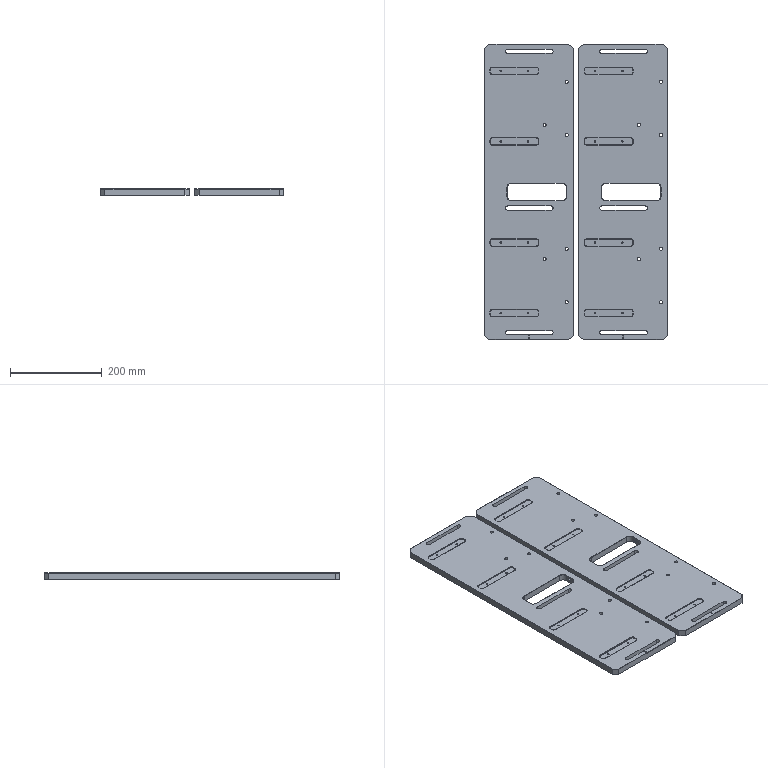NC program | NX | posted by the shop | part box 401 x 645 x 14 mm
Lines 2473 to 4203 of 5636, first 1379 of 1731 lines:
N3 T09 M06
(D10  D=10. R=0. H=09 ce=0.10 di=0.00)
G00 G90 G54 X0.0 Y205.6 M03 S6000
G43 H09 Z34.
M08
Z14.
G01 X312.5 Z13.907 F4000.
G02 X316.106 Y204.106 Z13.906 I0.0 J-5.1
G01 X326.106 Y194.106 Z13.902
G02 X327.6 Y190.5 Z13.901 I-3.606 J-3.606
G01 Y15.5 Z13.849
G02 X326.106 Y11.894 Z13.848 I-5.1 J0.0
G01 X316.106 Y1.894 Z13.844
G02 X312.5 Y.4 Z13.843 I-3.606 J3.606
G01 X-312.5 Z13.657
G02 X-316.106 Y1.894 Z13.656 I0.0 J5.1
G01 X-326.106 Y11.894 Z13.652
G02 X-327.6 Y15.5 Z13.651 I3.606 J3.606
G01 Y190.5 Z13.599
G02 X-327.596 Y190.713 Z13.599 I5.1 J0.0
X-326.106 Y194.106 Z13.598 I5.096 J-.213
G01 X-316.106 Y204.106 Z13.594
G02 X-312.5 Y205.6 Z13.593 I3.606 J-3.606
G01 X312.5 Z13.407
G02 X316.106 Y204.106 Z13.406 I0.0 J-5.1
G01 X326.106 Y194.106 Z13.402
G02 X327.6 Y190.5 Z13.401 I-3.606 J-3.606
G01 Y15.5 Z13.349
G02 X326.106 Y11.894 Z13.348 I-5.1 J0.0
G01 X316.106 Y1.894 Z13.344
G02 X312.5 Y.4 Z13.343 I-3.606 J3.606
G01 X-312.5 Z13.157
G02 X-316.106 Y1.894 Z13.156 I0.0 J5.1
G01 X-326.106 Y11.894 Z13.152
G02 X-327.6 Y15.5 Z13.151 I3.606 J3.606
G01 Y190.5 Z13.099
G02 X-327.596 Y190.713 Z13.099 I5.1 J0.0
X-326.106 Y194.106 Z13.098 I5.096 J-.213
G01 X-316.106 Y204.106 Z13.094
G02 X-312.5 Y205.6 Z13.093 I3.606 J-3.606
G01 X312.5 Z12.907
G02 X316.106 Y204.106 Z12.906 I0.0 J-5.1
G01 X326.106 Y194.106 Z12.902
G02 X327.6 Y190.5 Z12.901 I-3.606 J-3.606
G01 Y15.5 Z12.849
G02 X326.106 Y11.894 Z12.848 I-5.1 J0.0
G01 X316.106 Y1.894 Z12.844
G02 X312.5 Y.4 Z12.843 I-3.606 J3.606
G01 X-312.5 Z12.657
G02 X-316.106 Y1.894 Z12.656 I0.0 J5.1
G01 X-326.106 Y11.894 Z12.652
G02 X-327.6 Y15.5 Z12.651 I3.606 J3.606
G01 Y190.5 Z12.599
G02 X-327.596 Y190.713 Z12.599 I5.1 J0.0
X-326.106 Y194.106 Z12.598 I5.096 J-.213
G01 X-316.106 Y204.106 Z12.594
G02 X-312.5 Y205.6 Z12.593 I3.606 J-3.606
G01 X312.5 Z12.407
G02 X316.106 Y204.106 Z12.406 I0.0 J-5.1
G01 X326.106 Y194.106 Z12.402
G02 X327.6 Y190.5 Z12.401 I-3.606 J-3.606
G01 Y15.5 Z12.349
G02 X326.106 Y11.894 Z12.348 I-5.1 J0.0
G01 X316.106 Y1.894 Z12.344
G02 X312.5 Y.4 Z12.343 I-3.606 J3.606
G01 X-312.5 Z12.157
G02 X-316.106 Y1.894 Z12.156 I0.0 J5.1
G01 X-326.106 Y11.894 Z12.152
G02 X-327.6 Y15.5 Z12.151 I3.606 J3.606
G01 Y190.5 Z12.099
G02 X-327.596 Y190.713 Z12.099 I5.1 J0.0
X-326.106 Y194.106 Z12.098 I5.096 J-.213
G01 X-316.106 Y204.106 Z12.094
G02 X-312.5 Y205.6 Z12.093 I3.606 J-3.606
G01 X312.5 Z11.907
G02 X316.106 Y204.106 Z11.906 I0.0 J-5.1
G01 X326.106 Y194.106 Z11.902
G02 X327.6 Y190.5 Z11.901 I-3.606 J-3.606
G01 Y15.5 Z11.849
G02 X326.106 Y11.894 Z11.848 I-5.1 J0.0
G01 X316.106 Y1.894 Z11.844
G02 X312.5 Y.4 Z11.843 I-3.606 J3.606
G01 X-312.5 Z11.657
G02 X-316.106 Y1.894 Z11.656 I0.0 J5.1
G01 X-326.106 Y11.894 Z11.652
G02 X-327.6 Y15.5 Z11.651 I3.606 J3.606
G01 Y190.5 Z11.599
G02 X-327.596 Y190.713 Z11.599 I5.1 J0.0
X-326.106 Y194.106 Z11.598 I5.096 J-.213
G01 X-316.106 Y204.106 Z11.594
G02 X-312.5 Y205.6 Z11.593 I3.606 J-3.606
G01 X312.5 Z11.407
G02 X316.106 Y204.106 Z11.406 I0.0 J-5.1
G01 X326.106 Y194.106 Z11.402
G02 X327.6 Y190.5 Z11.401 I-3.606 J-3.606
G01 Y15.5 Z11.349
G02 X326.106 Y11.894 Z11.348 I-5.1 J0.0
G01 X316.106 Y1.894 Z11.344
G02 X312.5 Y.4 Z11.343 I-3.606 J3.606
G01 X-312.5 Z11.157
G02 X-316.106 Y1.894 Z11.156 I0.0 J5.1
G01 X-326.106 Y11.894 Z11.152
G02 X-327.6 Y15.5 Z11.151 I3.606 J3.606
G01 Y190.5 Z11.099
G02 X-327.596 Y190.713 Z11.099 I5.1 J0.0
X-326.106 Y194.106 Z11.098 I5.096 J-.213
G01 X-316.106 Y204.106 Z11.094
G02 X-312.5 Y205.6 Z11.093 I3.606 J-3.606
G01 X312.5 Z10.907
G02 X316.106 Y204.106 Z10.906 I0.0 J-5.1
G01 X326.106 Y194.106 Z10.902
G02 X327.6 Y190.5 Z10.901 I-3.606 J-3.606
G01 Y15.5 Z10.849
G02 X326.106 Y11.894 Z10.848 I-5.1 J0.0
G01 X316.106 Y1.894 Z10.844
G02 X312.5 Y.4 Z10.843 I-3.606 J3.606
G01 X-312.5 Z10.657
G02 X-316.106 Y1.894 Z10.656 I0.0 J5.1
G01 X-326.106 Y11.894 Z10.652
G02 X-327.6 Y15.5 Z10.651 I3.606 J3.606
G01 Y190.5 Z10.599
G02 X-327.596 Y190.713 Z10.599 I5.1 J0.0
X-326.106 Y194.106 Z10.598 I5.096 J-.213
G01 X-316.106 Y204.106 Z10.594
G02 X-312.5 Y205.6 Z10.593 I3.606 J-3.606
G01 X312.5 Z10.407
G02 X316.106 Y204.106 Z10.406 I0.0 J-5.1
G01 X326.106 Y194.106 Z10.402
G02 X327.6 Y190.5 Z10.401 I-3.606 J-3.606
G01 Y15.5 Z10.349
G02 X326.106 Y11.894 Z10.348 I-5.1 J0.0
G01 X316.106 Y1.894 Z10.344
G02 X312.5 Y.4 Z10.343 I-3.606 J3.606
G01 X-312.5 Z10.157
G02 X-316.106 Y1.894 Z10.156 I0.0 J5.1
G01 X-326.106 Y11.894 Z10.152
G02 X-327.6 Y15.5 Z10.151 I3.606 J3.606
G01 Y190.5 Z10.099
G02 X-327.596 Y190.713 Z10.099 I5.1 J0.0
X-326.106 Y194.106 Z10.098 I5.096 J-.213
G01 X-316.106 Y204.106 Z10.094
G02 X-312.5 Y205.6 Z10.093 I3.606 J-3.606
G01 X312.5 Z9.907
G02 X316.106 Y204.106 Z9.906 I0.0 J-5.1
G01 X326.106 Y194.106 Z9.902
G02 X327.6 Y190.5 Z9.901 I-3.606 J-3.606
G01 Y15.5 Z9.849
G02 X326.106 Y11.894 Z9.848 I-5.1 J0.0
G01 X316.106 Y1.894 Z9.844
G02 X312.5 Y.4 Z9.843 I-3.606 J3.606
G01 X-312.5 Z9.657
G02 X-316.106 Y1.894 Z9.656 I0.0 J5.1
G01 X-326.106 Y11.894 Z9.652
G02 X-327.6 Y15.5 Z9.651 I3.606 J3.606
G01 Y190.5 Z9.599
G02 X-327.596 Y190.713 Z9.599 I5.1 J0.0
X-326.106 Y194.106 Z9.598 I5.096 J-.213
G01 X-316.106 Y204.106 Z9.594
G02 X-312.5 Y205.6 Z9.593 I3.606 J-3.606
G01 X312.5 Z9.407
G02 X316.106 Y204.106 Z9.406 I0.0 J-5.1
G01 X326.106 Y194.106 Z9.402
G02 X327.6 Y190.5 Z9.401 I-3.606 J-3.606
G01 Y15.5 Z9.349
G02 X326.106 Y11.894 Z9.348 I-5.1 J0.0
G01 X316.106 Y1.894 Z9.344
G02 X312.5 Y.4 Z9.343 I-3.606 J3.606
G01 X-312.5 Z9.157
G02 X-316.106 Y1.894 Z9.156 I0.0 J5.1
G01 X-326.106 Y11.894 Z9.152
G02 X-327.6 Y15.5 Z9.151 I3.606 J3.606
G01 Y190.5 Z9.099
G02 X-327.596 Y190.713 Z9.099 I5.1 J0.0
X-326.106 Y194.106 Z9.098 I5.096 J-.213
G01 X-316.106 Y204.106 Z9.094
G02 X-312.5 Y205.6 Z9.093 I3.606 J-3.606
G01 X312.5 Z8.907
G02 X316.106 Y204.106 Z8.906 I0.0 J-5.1
G01 X326.106 Y194.106 Z8.902
G02 X327.6 Y190.5 Z8.901 I-3.606 J-3.606
G01 Y15.5 Z8.849
G02 X326.106 Y11.894 Z8.848 I-5.1 J0.0
G01 X316.106 Y1.894 Z8.844
G02 X312.5 Y.4 Z8.843 I-3.606 J3.606
G01 X-312.5 Z8.657
G02 X-316.106 Y1.894 Z8.656 I0.0 J5.1
G01 X-326.106 Y11.894 Z8.652
G02 X-327.6 Y15.5 Z8.651 I3.606 J3.606
G01 Y190.5 Z8.599
G02 X-327.596 Y190.713 Z8.599 I5.1 J0.0
X-326.106 Y194.106 Z8.598 I5.096 J-.213
G01 X-316.106 Y204.106 Z8.594
G02 X-312.5 Y205.6 Z8.593 I3.606 J-3.606
G01 X312.5 Z8.407
G02 X316.106 Y204.106 Z8.406 I0.0 J-5.1
G01 X326.106 Y194.106 Z8.402
G02 X327.6 Y190.5 Z8.401 I-3.606 J-3.606
G01 Y15.5 Z8.349
G02 X326.106 Y11.894 Z8.348 I-5.1 J0.0
G01 X316.106 Y1.894 Z8.344
G02 X312.5 Y.4 Z8.343 I-3.606 J3.606
G01 X-312.5 Z8.157
G02 X-316.106 Y1.894 Z8.156 I0.0 J5.1
G01 X-326.106 Y11.894 Z8.152
G02 X-327.6 Y15.5 Z8.151 I3.606 J3.606
G01 Y190.5 Z8.099
G02 X-327.596 Y190.713 Z8.099 I5.1 J0.0
X-326.106 Y194.106 Z8.098 I5.096 J-.213
G01 X-316.106 Y204.106 Z8.094
G02 X-312.5 Y205.6 Z8.093 I3.606 J-3.606
G01 X312.5 Z7.907
G02 X316.106 Y204.106 Z7.906 I0.0 J-5.1
G01 X326.106 Y194.106 Z7.902
G02 X327.6 Y190.5 Z7.901 I-3.606 J-3.606
G01 Y15.5 Z7.849
G02 X326.106 Y11.894 Z7.848 I-5.1 J0.0
G01 X316.106 Y1.894 Z7.844
G02 X312.5 Y.4 Z7.843 I-3.606 J3.606
G01 X-312.5 Z7.657
G02 X-316.106 Y1.894 Z7.656 I0.0 J5.1
G01 X-326.106 Y11.894 Z7.652
G02 X-327.6 Y15.5 Z7.651 I3.606 J3.606
G01 Y190.5 Z7.599
G02 X-327.596 Y190.713 Z7.599 I5.1 J0.0
X-326.106 Y194.106 Z7.598 I5.096 J-.213
G01 X-316.106 Y204.106 Z7.594
G02 X-312.5 Y205.6 Z7.593 I3.606 J-3.606
G01 X312.5 Z7.407
G02 X316.106 Y204.106 Z7.406 I0.0 J-5.1
G01 X326.106 Y194.106 Z7.402
G02 X327.6 Y190.5 Z7.401 I-3.606 J-3.606
G01 Y15.5 Z7.349
G02 X326.106 Y11.894 Z7.348 I-5.1 J0.0
G01 X316.106 Y1.894 Z7.344
G02 X312.5 Y.4 Z7.343 I-3.606 J3.606
G01 X-312.5 Z7.157
G02 X-316.106 Y1.894 Z7.156 I0.0 J5.1
G01 X-326.106 Y11.894 Z7.152
G02 X-327.6 Y15.5 Z7.151 I3.606 J3.606
G01 Y190.5 Z7.099
G02 X-327.596 Y190.713 Z7.099 I5.1 J0.0
X-326.106 Y194.106 Z7.098 I5.096 J-.213
G01 X-316.106 Y204.106 Z7.094
G02 X-312.5 Y205.6 Z7.093 I3.606 J-3.606
G01 X312.5 Z6.907
G02 X316.106 Y204.106 Z6.906 I0.0 J-5.1
G01 X326.106 Y194.106 Z6.902
G02 X327.6 Y190.5 Z6.901 I-3.606 J-3.606
G01 Y15.5 Z6.849
G02 X326.106 Y11.894 Z6.848 I-5.1 J0.0
G01 X316.106 Y1.894 Z6.844
G02 X312.5 Y.4 Z6.843 I-3.606 J3.606
G01 X-312.5 Z6.657
G02 X-316.106 Y1.894 Z6.656 I0.0 J5.1
G01 X-326.106 Y11.894 Z6.652
G02 X-327.6 Y15.5 Z6.651 I3.606 J3.606
G01 Y190.5 Z6.599
G02 X-327.596 Y190.713 Z6.599 I5.1 J0.0
X-326.106 Y194.106 Z6.598 I5.096 J-.213
G01 X-316.106 Y204.106 Z6.594
G02 X-312.5 Y205.6 Z6.593 I3.606 J-3.606
G01 X312.5 Z6.407
G02 X316.106 Y204.106 Z6.406 I0.0 J-5.1
G01 X326.106 Y194.106 Z6.402
G02 X327.6 Y190.5 Z6.401 I-3.606 J-3.606
G01 Y15.5 Z6.349
G02 X326.106 Y11.894 Z6.348 I-5.1 J0.0
G01 X316.106 Y1.894 Z6.344
G02 X312.5 Y.4 Z6.343 I-3.606 J3.606
G01 X-312.5 Z6.157
G02 X-316.106 Y1.894 Z6.156 I0.0 J5.1
G01 X-326.106 Y11.894 Z6.152
G02 X-327.6 Y15.5 Z6.151 I3.606 J3.606
G01 Y190.5 Z6.099
G02 X-327.596 Y190.713 Z6.099 I5.1 J0.0
X-326.106 Y194.106 Z6.098 I5.096 J-.213
G01 X-316.106 Y204.106 Z6.094
G02 X-312.5 Y205.6 Z6.093 I3.606 J-3.606
G01 X312.5 Z5.907
G02 X316.106 Y204.106 Z5.906 I0.0 J-5.1
G01 X326.106 Y194.106 Z5.902
G02 X327.6 Y190.5 Z5.901 I-3.606 J-3.606
G01 Y15.5 Z5.849
G02 X326.106 Y11.894 Z5.848 I-5.1 J0.0
G01 X316.106 Y1.894 Z5.844
G02 X312.5 Y.4 Z5.843 I-3.606 J3.606
G01 X-312.5 Z5.657
G02 X-316.106 Y1.894 Z5.656 I0.0 J5.1
G01 X-326.106 Y11.894 Z5.652
G02 X-327.6 Y15.5 Z5.651 I3.606 J3.606
G01 Y190.5 Z5.599
G02 X-327.596 Y190.713 Z5.599 I5.1 J0.0
X-326.106 Y194.106 Z5.598 I5.096 J-.213
G01 X-316.106 Y204.106 Z5.594
G02 X-312.5 Y205.6 Z5.593 I3.606 J-3.606
G01 X312.5 Z5.407
G02 X316.106 Y204.106 Z5.406 I0.0 J-5.1
G01 X326.106 Y194.106 Z5.402
G02 X327.6 Y190.5 Z5.401 I-3.606 J-3.606
G01 Y15.5 Z5.349
G02 X326.106 Y11.894 Z5.348 I-5.1 J0.0
G01 X316.106 Y1.894 Z5.344
G02 X312.5 Y.4 Z5.343 I-3.606 J3.606
G01 X-312.5 Z5.157
G02 X-316.106 Y1.894 Z5.156 I0.0 J5.1
G01 X-326.106 Y11.894 Z5.152
G02 X-327.6 Y15.5 Z5.151 I3.606 J3.606
G01 Y190.5 Z5.099
G02 X-327.596 Y190.713 Z5.099 I5.1 J0.0
X-326.106 Y194.106 Z5.098 I5.096 J-.213
G01 X-316.106 Y204.106 Z5.094
G02 X-312.5 Y205.6 Z5.093 I3.606 J-3.606
G01 X312.5 Z4.907
G02 X316.106 Y204.106 Z4.906 I0.0 J-5.1
G01 X326.106 Y194.106 Z4.902
G02 X327.6 Y190.5 Z4.901 I-3.606 J-3.606
G01 Y15.5 Z4.849
G02 X326.106 Y11.894 Z4.848 I-5.1 J0.0
G01 X316.106 Y1.894 Z4.844
G02 X312.5 Y.4 Z4.843 I-3.606 J3.606
G01 X-312.5 Z4.657
G02 X-316.106 Y1.894 Z4.656 I0.0 J5.1
G01 X-326.106 Y11.894 Z4.652
G02 X-327.6 Y15.5 Z4.651 I3.606 J3.606
G01 Y190.5 Z4.599
G02 X-327.596 Y190.713 Z4.599 I5.1 J0.0
X-326.106 Y194.106 Z4.598 I5.096 J-.213
G01 X-316.106 Y204.106 Z4.594
G02 X-312.5 Y205.6 Z4.593 I3.606 J-3.606
G01 X312.5 Z4.407
G02 X316.106 Y204.106 Z4.406 I0.0 J-5.1
G01 X326.106 Y194.106 Z4.402
G02 X327.6 Y190.5 Z4.401 I-3.606 J-3.606
G01 Y15.5 Z4.349
G02 X326.106 Y11.894 Z4.348 I-5.1 J0.0
G01 X316.106 Y1.894 Z4.344
G02 X312.5 Y.4 Z4.343 I-3.606 J3.606
G01 X-312.5 Z4.157
G02 X-316.106 Y1.894 Z4.156 I0.0 J5.1
G01 X-326.106 Y11.894 Z4.152
G02 X-327.6 Y15.5 Z4.151 I3.606 J3.606
G01 Y190.5 Z4.099
G02 X-327.596 Y190.713 Z4.099 I5.1 J0.0
X-326.106 Y194.106 Z4.098 I5.096 J-.213
G01 X-316.106 Y204.106 Z4.094
G02 X-312.5 Y205.6 Z4.093 I3.606 J-3.606
G01 X312.5 Z3.907
G02 X316.106 Y204.106 Z3.906 I0.0 J-5.1
G01 X326.106 Y194.106 Z3.902
G02 X327.6 Y190.5 Z3.901 I-3.606 J-3.606
G01 Y15.5 Z3.849
G02 X326.106 Y11.894 Z3.848 I-5.1 J0.0
G01 X316.106 Y1.894 Z3.844
G02 X312.5 Y.4 Z3.843 I-3.606 J3.606
G01 X-312.5 Z3.657
G02 X-316.106 Y1.894 Z3.656 I0.0 J5.1
G01 X-326.106 Y11.894 Z3.652
G02 X-327.6 Y15.5 Z3.651 I3.606 J3.606
G01 Y190.5 Z3.599
G02 X-327.596 Y190.713 Z3.599 I5.1 J0.0
X-326.106 Y194.106 Z3.598 I5.096 J-.213
G01 X-316.106 Y204.106 Z3.594
G02 X-312.5 Y205.6 Z3.593 I3.606 J-3.606
G01 X312.5 Z3.407
G02 X316.106 Y204.106 Z3.406 I0.0 J-5.1
G01 X326.106 Y194.106 Z3.402
G02 X327.6 Y190.5 Z3.401 I-3.606 J-3.606
G01 Y15.5 Z3.349
G02 X326.106 Y11.894 Z3.348 I-5.1 J0.0
G01 X316.106 Y1.894 Z3.344
G02 X312.5 Y.4 Z3.343 I-3.606 J3.606
G01 X-312.5 Z3.157
G02 X-316.106 Y1.894 Z3.156 I0.0 J5.1
G01 X-326.106 Y11.894 Z3.152
G02 X-327.6 Y15.5 Z3.151 I3.606 J3.606
G01 Y190.5 Z3.099
G02 X-327.596 Y190.713 Z3.099 I5.1 J0.0
X-326.106 Y194.106 Z3.098 I5.096 J-.213
G01 X-316.106 Y204.106 Z3.094
G02 X-312.5 Y205.6 Z3.093 I3.606 J-3.606
G01 X312.5 Z2.907
G02 X316.106 Y204.106 Z2.906 I0.0 J-5.1
G01 X326.106 Y194.106 Z2.902
G02 X327.6 Y190.5 Z2.901 I-3.606 J-3.606
G01 Y15.5 Z2.849
G02 X326.106 Y11.894 Z2.848 I-5.1 J0.0
G01 X316.106 Y1.894 Z2.844
G02 X312.5 Y.4 Z2.843 I-3.606 J3.606
G01 X-312.5 Z2.657
G02 X-316.106 Y1.894 Z2.656 I0.0 J5.1
G01 X-326.106 Y11.894 Z2.652
G02 X-327.6 Y15.5 Z2.651 I3.606 J3.606
G01 Y190.5 Z2.599
G02 X-327.596 Y190.713 Z2.599 I5.1 J0.0
X-326.106 Y194.106 Z2.598 I5.096 J-.213
G01 X-316.106 Y204.106 Z2.594
G02 X-312.5 Y205.6 Z2.593 I3.606 J-3.606
G01 X312.5 Z2.407
G02 X316.106 Y204.106 Z2.406 I0.0 J-5.1
G01 X326.106 Y194.106 Z2.402
G02 X327.6 Y190.5 Z2.401 I-3.606 J-3.606
G01 Y15.5 Z2.349
G02 X326.106 Y11.894 Z2.348 I-5.1 J0.0
G01 X316.106 Y1.894 Z2.344
G02 X312.5 Y.4 Z2.343 I-3.606 J3.606
G01 X-312.5 Z2.157
G02 X-316.106 Y1.894 Z2.156 I0.0 J5.1
G01 X-326.106 Y11.894 Z2.152
G02 X-327.6 Y15.5 Z2.151 I3.606 J3.606
G01 Y190.5 Z2.099
G02 X-327.596 Y190.713 Z2.099 I5.1 J0.0
X-326.106 Y194.106 Z2.098 I5.096 J-.213
G01 X-316.106 Y204.106 Z2.094
G02 X-312.5 Y205.6 Z2.093 I3.606 J-3.606
G01 X312.5 Z1.907
G02 X316.106 Y204.106 Z1.906 I0.0 J-5.1
G01 X326.106 Y194.106 Z1.902
G02 X327.6 Y190.5 Z1.901 I-3.606 J-3.606
G01 Y15.5 Z1.849
G02 X326.106 Y11.894 Z1.848 I-5.1 J0.0
G01 X316.106 Y1.894 Z1.844
G02 X312.5 Y.4 Z1.843 I-3.606 J3.606
G01 X-312.5 Z1.657
G02 X-316.106 Y1.894 Z1.656 I0.0 J5.1
G01 X-326.106 Y11.894 Z1.652
G02 X-327.6 Y15.5 Z1.651 I3.606 J3.606
G01 Y190.5 Z1.599
G02 X-327.596 Y190.713 Z1.599 I5.1 J0.0
X-326.106 Y194.106 Z1.598 I5.096 J-.213
G01 X-316.106 Y204.106 Z1.594
G02 X-312.5 Y205.6 Z1.593 I3.606 J-3.606
G01 X312.5 Z1.407
G02 X316.106 Y204.106 Z1.406 I0.0 J-5.1
G01 X326.106 Y194.106 Z1.402
G02 X327.6 Y190.5 Z1.401 I-3.606 J-3.606
G01 Y15.5 Z1.349
G02 X326.106 Y11.894 Z1.348 I-5.1 J0.0
G01 X316.106 Y1.894 Z1.344
G02 X312.5 Y.4 Z1.343 I-3.606 J3.606
G01 X-312.5 Z1.157
G02 X-316.106 Y1.894 Z1.156 I0.0 J5.1
G01 X-326.106 Y11.894 Z1.152
G02 X-327.6 Y15.5 Z1.151 I3.606 J3.606
G01 Y190.5 Z1.099
G02 X-327.596 Y190.713 Z1.099 I5.1 J0.0
X-326.106 Y194.106 Z1.098 I5.096 J-.213
G01 X-316.106 Y204.106 Z1.094
G02 X-312.5 Y205.6 Z1.093 I3.606 J-3.606
G01 X312.5 Z.907
G02 X316.106 Y204.106 Z.906 I0.0 J-5.1
G01 X326.106 Y194.106 Z.902
G02 X327.6 Y190.5 Z.901 I-3.606 J-3.606
G01 Y15.5 Z.849
G02 X326.106 Y11.894 Z.848 I-5.1 J0.0
G01 X316.106 Y1.894 Z.844
G02 X312.5 Y.4 Z.843 I-3.606 J3.606
G01 X-312.5 Z.657
G02 X-316.106 Y1.894 Z.656 I0.0 J5.1
G01 X-326.106 Y11.894 Z.652
G02 X-327.6 Y15.5 Z.651 I3.606 J3.606
G01 Y190.5 Z.599
G02 X-327.596 Y190.713 Z.599 I5.1 J0.0
X-326.106 Y194.106 Z.598 I5.096 J-.213
G01 X-316.106 Y204.106 Z.594
G02 X-312.5 Y205.6 Z.593 I3.606 J-3.606
G01 X0.0 Z.5
X312.5
G02 X316.106 Y204.106 I0.0 J-5.1
G01 X326.106 Y194.106
G02 X327.6 Y190.5 I-3.606 J-3.606
G01 Y15.5
G02 X326.106 Y11.894 I-5.1 J0.0
G01 X316.106 Y1.894
G02 X312.5 Y.4 I-3.606 J3.606
G01 X-312.5
G02 X-316.106 Y1.894 I0.0 J5.1
G01 X-326.106 Y11.894
G02 X-327.6 Y15.5 I3.606 J3.606
G01 Y190.5
G02 X-326.106 Y194.106 I5.1 J0.0
G01 X-316.106 Y204.106
G02 X-312.5 Y205.6 I3.606 J-3.606
G01 X0.0
X.5
Z1.5
G00 Z34.
X0.0 Y-205.6
Z14.
G01 X-312.5 Z13.907
G02 X-316.106 Y-204.106 Z13.906 I0.0 J5.1
G01 X-326.106 Y-194.106 Z13.902
G02 X-327.6 Y-190.5 Z13.901 I3.606 J3.606
G01 Y-15.5 Z13.849
G02 X-326.106 Y-11.894 Z13.848 I5.1 J0.0
G01 X-316.106 Y-1.894 Z13.844
G02 X-312.5 Y-.4 Z13.843 I3.606 J-3.606
G01 X312.5 Z13.657
G02 X316.106 Y-1.894 Z13.656 I0.0 J-5.1
G01 X326.106 Y-11.894 Z13.652
G02 X327.6 Y-15.5 Z13.651 I-3.606 J-3.606
G01 Y-190.5 Z13.599
G02 X326.106 Y-194.106 Z13.598 I-5.1 J0.0
G01 X316.106 Y-204.106 Z13.594
G02 X312.5 Y-205.6 Z13.593 I-3.606 J3.606
G01 X-312.5 Z13.407
G02 X-316.106 Y-204.106 Z13.406 I0.0 J5.1
G01 X-326.106 Y-194.106 Z13.402
G02 X-327.6 Y-190.5 Z13.401 I3.606 J3.606
G01 Y-15.5 Z13.349
G02 X-326.106 Y-11.894 Z13.348 I5.1 J0.0
G01 X-316.106 Y-1.894 Z13.344
G02 X-312.5 Y-.4 Z13.343 I3.606 J-3.606
G01 X312.5 Z13.157
G02 X316.106 Y-1.894 Z13.156 I0.0 J-5.1
G01 X326.106 Y-11.894 Z13.152
G02 X327.6 Y-15.5 Z13.151 I-3.606 J-3.606
G01 Y-190.5 Z13.099
G02 X326.106 Y-194.106 Z13.098 I-5.1 J0.0
G01 X316.106 Y-204.106 Z13.094
G02 X312.5 Y-205.6 Z13.093 I-3.606 J3.606
G01 X-312.5 Z12.907
G02 X-316.106 Y-204.106 Z12.906 I0.0 J5.1
G01 X-326.106 Y-194.106 Z12.902
G02 X-327.6 Y-190.5 Z12.901 I3.606 J3.606
G01 Y-15.5 Z12.849
G02 X-326.106 Y-11.894 Z12.848 I5.1 J0.0
G01 X-316.106 Y-1.894 Z12.844
G02 X-312.5 Y-.4 Z12.843 I3.606 J-3.606
G01 X312.5 Z12.657
G02 X316.106 Y-1.894 Z12.656 I0.0 J-5.1
G01 X326.106 Y-11.894 Z12.652
G02 X327.6 Y-15.5 Z12.651 I-3.606 J-3.606
G01 Y-190.5 Z12.599
G02 X326.106 Y-194.106 Z12.598 I-5.1 J0.0
G01 X316.106 Y-204.106 Z12.594
G02 X312.5 Y-205.6 Z12.593 I-3.606 J3.606
G01 X-312.5 Z12.407
G02 X-316.106 Y-204.106 Z12.406 I0.0 J5.1
G01 X-326.106 Y-194.106 Z12.402
G02 X-327.6 Y-190.5 Z12.401 I3.606 J3.606
G01 Y-15.5 Z12.349
G02 X-326.106 Y-11.894 Z12.348 I5.1 J0.0
G01 X-316.106 Y-1.894 Z12.344
G02 X-312.5 Y-.4 Z12.343 I3.606 J-3.606
G01 X312.5 Z12.157
G02 X316.106 Y-1.894 Z12.156 I0.0 J-5.1
G01 X326.106 Y-11.894 Z12.152
G02 X327.6 Y-15.5 Z12.151 I-3.606 J-3.606
G01 Y-190.5 Z12.099
G02 X326.106 Y-194.106 Z12.098 I-5.1 J0.0
G01 X316.106 Y-204.106 Z12.094
G02 X312.5 Y-205.6 Z12.093 I-3.606 J3.606
G01 X-312.5 Z11.907
G02 X-316.106 Y-204.106 Z11.906 I0.0 J5.1
G01 X-326.106 Y-194.106 Z11.902
G02 X-327.6 Y-190.5 Z11.901 I3.606 J3.606
G01 Y-15.5 Z11.849
G02 X-326.106 Y-11.894 Z11.848 I5.1 J0.0
G01 X-316.106 Y-1.894 Z11.844
G02 X-312.5 Y-.4 Z11.843 I3.606 J-3.606
G01 X312.5 Z11.657
G02 X316.106 Y-1.894 Z11.656 I0.0 J-5.1
G01 X326.106 Y-11.894 Z11.652
G02 X327.6 Y-15.5 Z11.651 I-3.606 J-3.606
G01 Y-190.5 Z11.599
G02 X326.106 Y-194.106 Z11.598 I-5.1 J0.0
G01 X316.106 Y-204.106 Z11.594
G02 X312.5 Y-205.6 Z11.593 I-3.606 J3.606
G01 X-312.5 Z11.407
G02 X-316.106 Y-204.106 Z11.406 I0.0 J5.1
G01 X-326.106 Y-194.106 Z11.402
G02 X-327.6 Y-190.5 Z11.401 I3.606 J3.606
G01 Y-15.5 Z11.349
G02 X-326.106 Y-11.894 Z11.348 I5.1 J0.0
G01 X-316.106 Y-1.894 Z11.344
G02 X-312.5 Y-.4 Z11.343 I3.606 J-3.606
G01 X312.5 Z11.157
G02 X316.106 Y-1.894 Z11.156 I0.0 J-5.1
G01 X326.106 Y-11.894 Z11.152
G02 X327.6 Y-15.5 Z11.151 I-3.606 J-3.606
G01 Y-190.5 Z11.099
G02 X326.106 Y-194.106 Z11.098 I-5.1 J0.0
G01 X316.106 Y-204.106 Z11.094
G02 X312.5 Y-205.6 Z11.093 I-3.606 J3.606
G01 X-312.5 Z10.907
G02 X-316.106 Y-204.106 Z10.906 I0.0 J5.1
G01 X-326.106 Y-194.106 Z10.902
G02 X-327.6 Y-190.5 Z10.901 I3.606 J3.606
G01 Y-15.5 Z10.849
G02 X-326.106 Y-11.894 Z10.848 I5.1 J0.0
G01 X-316.106 Y-1.894 Z10.844
G02 X-312.5 Y-.4 Z10.843 I3.606 J-3.606
G01 X312.5 Z10.657
G02 X316.106 Y-1.894 Z10.656 I0.0 J-5.1
G01 X326.106 Y-11.894 Z10.652
G02 X327.6 Y-15.5 Z10.651 I-3.606 J-3.606
G01 Y-190.5 Z10.599
G02 X326.106 Y-194.106 Z10.598 I-5.1 J0.0
G01 X316.106 Y-204.106 Z10.594
G02 X312.5 Y-205.6 Z10.593 I-3.606 J3.606
G01 X-312.5 Z10.407
G02 X-316.106 Y-204.106 Z10.406 I0.0 J5.1
G01 X-326.106 Y-194.106 Z10.402
G02 X-327.6 Y-190.5 Z10.401 I3.606 J3.606
G01 Y-15.5 Z10.349
G02 X-326.106 Y-11.894 Z10.348 I5.1 J0.0
G01 X-316.106 Y-1.894 Z10.344
G02 X-312.5 Y-.4 Z10.343 I3.606 J-3.606
G01 X312.5 Z10.157
G02 X316.106 Y-1.894 Z10.156 I0.0 J-5.1
G01 X326.106 Y-11.894 Z10.152
G02 X327.6 Y-15.5 Z10.151 I-3.606 J-3.606
G01 Y-190.5 Z10.099
G02 X326.106 Y-194.106 Z10.098 I-5.1 J0.0
G01 X316.106 Y-204.106 Z10.094
G02 X312.5 Y-205.6 Z10.093 I-3.606 J3.606
G01 X-312.5 Z9.907
G02 X-316.106 Y-204.106 Z9.906 I0.0 J5.1
G01 X-326.106 Y-194.106 Z9.902
G02 X-327.6 Y-190.5 Z9.901 I3.606 J3.606
G01 Y-15.5 Z9.849
G02 X-326.106 Y-11.894 Z9.848 I5.1 J0.0
G01 X-316.106 Y-1.894 Z9.844
G02 X-312.5 Y-.4 Z9.843 I3.606 J-3.606
G01 X312.5 Z9.657
G02 X316.106 Y-1.894 Z9.656 I0.0 J-5.1
G01 X326.106 Y-11.894 Z9.652
G02 X327.6 Y-15.5 Z9.651 I-3.606 J-3.606
G01 Y-190.5 Z9.599
G02 X326.106 Y-194.106 Z9.598 I-5.1 J0.0
G01 X316.106 Y-204.106 Z9.594
G02 X312.5 Y-205.6 Z9.593 I-3.606 J3.606
G01 X-312.5 Z9.407
G02 X-316.106 Y-204.106 Z9.406 I0.0 J5.1
G01 X-326.106 Y-194.106 Z9.402
G02 X-327.6 Y-190.5 Z9.401 I3.606 J3.606
G01 Y-15.5 Z9.349
G02 X-326.106 Y-11.894 Z9.348 I5.1 J0.0
G01 X-316.106 Y-1.894 Z9.344
G02 X-312.5 Y-.4 Z9.343 I3.606 J-3.606
G01 X312.5 Z9.157
G02 X316.106 Y-1.894 Z9.156 I0.0 J-5.1
G01 X326.106 Y-11.894 Z9.152
G02 X327.6 Y-15.5 Z9.151 I-3.606 J-3.606
G01 Y-190.5 Z9.099
G02 X326.106 Y-194.106 Z9.098 I-5.1 J0.0
G01 X316.106 Y-204.106 Z9.094
G02 X312.5 Y-205.6 Z9.093 I-3.606 J3.606
G01 X-312.5 Z8.907
G02 X-316.106 Y-204.106 Z8.906 I0.0 J5.1
G01 X-326.106 Y-194.106 Z8.902
G02 X-327.6 Y-190.5 Z8.901 I3.606 J3.606
G01 Y-15.5 Z8.849
G02 X-326.106 Y-11.894 Z8.848 I5.1 J0.0
G01 X-316.106 Y-1.894 Z8.844
G02 X-312.5 Y-.4 Z8.843 I3.606 J-3.606
G01 X312.5 Z8.657
G02 X316.106 Y-1.894 Z8.656 I0.0 J-5.1
G01 X326.106 Y-11.894 Z8.652
G02 X327.6 Y-15.5 Z8.651 I-3.606 J-3.606
G01 Y-190.5 Z8.599
G02 X326.106 Y-194.106 Z8.598 I-5.1 J0.0
G01 X316.106 Y-204.106 Z8.594
G02 X312.5 Y-205.6 Z8.593 I-3.606 J3.606
G01 X-312.5 Z8.407
G02 X-316.106 Y-204.106 Z8.406 I0.0 J5.1
G01 X-326.106 Y-194.106 Z8.402
G02 X-327.6 Y-190.5 Z8.401 I3.606 J3.606
G01 Y-15.5 Z8.349
G02 X-326.106 Y-11.894 Z8.348 I5.1 J0.0
G01 X-316.106 Y-1.894 Z8.344
G02 X-312.5 Y-.4 Z8.343 I3.606 J-3.606
G01 X312.5 Z8.157
G02 X316.106 Y-1.894 Z8.156 I0.0 J-5.1
G01 X326.106 Y-11.894 Z8.152
G02 X327.6 Y-15.5 Z8.151 I-3.606 J-3.606
G01 Y-190.5 Z8.099
G02 X326.106 Y-194.106 Z8.098 I-5.1 J0.0
G01 X316.106 Y-204.106 Z8.094
G02 X312.5 Y-205.6 Z8.093 I-3.606 J3.606
G01 X-312.5 Z7.907
G02 X-316.106 Y-204.106 Z7.906 I0.0 J5.1
G01 X-326.106 Y-194.106 Z7.902
G02 X-327.6 Y-190.5 Z7.901 I3.606 J3.606
G01 Y-15.5 Z7.849
G02 X-326.106 Y-11.894 Z7.848 I5.1 J0.0
G01 X-316.106 Y-1.894 Z7.844
G02 X-312.5 Y-.4 Z7.843 I3.606 J-3.606
G01 X312.5 Z7.657
G02 X316.106 Y-1.894 Z7.656 I0.0 J-5.1
G01 X326.106 Y-11.894 Z7.652
G02 X327.6 Y-15.5 Z7.651 I-3.606 J-3.606
G01 Y-190.5 Z7.599
G02 X326.106 Y-194.106 Z7.598 I-5.1 J0.0
G01 X316.106 Y-204.106 Z7.594
G02 X312.5 Y-205.6 Z7.593 I-3.606 J3.606
G01 X-312.5 Z7.407
G02 X-316.106 Y-204.106 Z7.406 I0.0 J5.1
G01 X-326.106 Y-194.106 Z7.402
G02 X-327.6 Y-190.5 Z7.401 I3.606 J3.606
G01 Y-15.5 Z7.349
G02 X-326.106 Y-11.894 Z7.348 I5.1 J0.0
G01 X-316.106 Y-1.894 Z7.344
G02 X-312.5 Y-.4 Z7.343 I3.606 J-3.606
G01 X312.5 Z7.157
G02 X316.106 Y-1.894 Z7.156 I0.0 J-5.1
G01 X326.106 Y-11.894 Z7.152
G02 X327.6 Y-15.5 Z7.151 I-3.606 J-3.606
G01 Y-190.5 Z7.099
G02 X326.106 Y-194.106 Z7.098 I-5.1 J0.0
G01 X316.106 Y-204.106 Z7.094
G02 X312.5 Y-205.6 Z7.093 I-3.606 J3.606
G01 X-312.5 Z6.907
G02 X-316.106 Y-204.106 Z6.906 I0.0 J5.1
G01 X-326.106 Y-194.106 Z6.902
G02 X-327.6 Y-190.5 Z6.901 I3.606 J3.606
G01 Y-15.5 Z6.849
G02 X-326.106 Y-11.894 Z6.848 I5.1 J0.0
G01 X-316.106 Y-1.894 Z6.844
G02 X-312.5 Y-.4 Z6.843 I3.606 J-3.606
G01 X312.5 Z6.657
G02 X316.106 Y-1.894 Z6.656 I0.0 J-5.1
G01 X326.106 Y-11.894 Z6.652
G02 X327.6 Y-15.5 Z6.651 I-3.606 J-3.606
G01 Y-190.5 Z6.599
G02 X326.106 Y-194.106 Z6.598 I-5.1 J0.0
G01 X316.106 Y-204.106 Z6.594
G02 X312.5 Y-205.6 Z6.593 I-3.606 J3.606
G01 X-312.5 Z6.407
G02 X-316.106 Y-204.106 Z6.406 I0.0 J5.1
G01 X-326.106 Y-194.106 Z6.402
G02 X-327.6 Y-190.5 Z6.401 I3.606 J3.606
G01 Y-15.5 Z6.349
G02 X-326.106 Y-11.894 Z6.348 I5.1 J0.0
G01 X-316.106 Y-1.894 Z6.344
G02 X-312.5 Y-.4 Z6.343 I3.606 J-3.606
G01 X312.5 Z6.157
G02 X316.106 Y-1.894 Z6.156 I0.0 J-5.1
G01 X326.106 Y-11.894 Z6.152
G02 X327.6 Y-15.5 Z6.151 I-3.606 J-3.606
G01 Y-190.5 Z6.099
G02 X326.106 Y-194.106 Z6.098 I-5.1 J0.0
G01 X316.106 Y-204.106 Z6.094
G02 X312.5 Y-205.6 Z6.093 I-3.606 J3.606
G01 X-312.5 Z5.907
G02 X-316.106 Y-204.106 Z5.906 I0.0 J5.1
G01 X-326.106 Y-194.106 Z5.902
G02 X-327.6 Y-190.5 Z5.901 I3.606 J3.606
G01 Y-15.5 Z5.849
G02 X-326.106 Y-11.894 Z5.848 I5.1 J0.0
G01 X-316.106 Y-1.894 Z5.844
G02 X-312.5 Y-.4 Z5.843 I3.606 J-3.606
G01 X312.5 Z5.657
G02 X316.106 Y-1.894 Z5.656 I0.0 J-5.1
G01 X326.106 Y-11.894 Z5.652
G02 X327.6 Y-15.5 Z5.651 I-3.606 J-3.606
G01 Y-190.5 Z5.599
G02 X326.106 Y-194.106 Z5.598 I-5.1 J0.0
G01 X316.106 Y-204.106 Z5.594
G02 X312.5 Y-205.6 Z5.593 I-3.606 J3.606
G01 X-312.5 Z5.407
G02 X-316.106 Y-204.106 Z5.406 I0.0 J5.1
G01 X-326.106 Y-194.106 Z5.402
G02 X-327.6 Y-190.5 Z5.401 I3.606 J3.606
G01 Y-15.5 Z5.349
G02 X-326.106 Y-11.894 Z5.348 I5.1 J0.0
G01 X-316.106 Y-1.894 Z5.344
G02 X-312.5 Y-.4 Z5.343 I3.606 J-3.606
G01 X312.5 Z5.157
G02 X316.106 Y-1.894 Z5.156 I0.0 J-5.1
G01 X326.106 Y-11.894 Z5.152
G02 X327.6 Y-15.5 Z5.151 I-3.606 J-3.606
G01 Y-190.5 Z5.099
G02 X326.106 Y-194.106 Z5.098 I-5.1 J0.0
G01 X316.106 Y-204.106 Z5.094
G02 X312.5 Y-205.6 Z5.093 I-3.606 J3.606
G01 X-312.5 Z4.907
G02 X-316.106 Y-204.106 Z4.906 I0.0 J5.1
G01 X-326.106 Y-194.106 Z4.902
G02 X-327.6 Y-190.5 Z4.901 I3.606 J3.606
G01 Y-15.5 Z4.849
G02 X-326.106 Y-11.894 Z4.848 I5.1 J0.0
G01 X-316.106 Y-1.894 Z4.844
G02 X-312.5 Y-.4 Z4.843 I3.606 J-3.606
G01 X312.5 Z4.657
G02 X316.106 Y-1.894 Z4.656 I0.0 J-5.1
G01 X326.106 Y-11.894 Z4.652
G02 X327.6 Y-15.5 Z4.651 I-3.606 J-3.606
G01 Y-190.5 Z4.599
G02 X326.106 Y-194.106 Z4.598 I-5.1 J0.0
G01 X316.106 Y-204.106 Z4.594
G02 X312.5 Y-205.6 Z4.593 I-3.606 J3.606
G01 X-312.5 Z4.407
G02 X-316.106 Y-204.106 Z4.406 I0.0 J5.1
G01 X-326.106 Y-194.106 Z4.402
G02 X-327.6 Y-190.5 Z4.401 I3.606 J3.606
G01 Y-15.5 Z4.349
G02 X-326.106 Y-11.894 Z4.348 I5.1 J0.0
G01 X-316.106 Y-1.894 Z4.344
G02 X-312.5 Y-.4 Z4.343 I3.606 J-3.606
G01 X312.5 Z4.157
G02 X316.106 Y-1.894 Z4.156 I0.0 J-5.1
G01 X326.106 Y-11.894 Z4.152
G02 X327.6 Y-15.5 Z4.151 I-3.606 J-3.606
G01 Y-190.5 Z4.099
G02 X326.106 Y-194.106 Z4.098 I-5.1 J0.0
G01 X316.106 Y-204.106 Z4.094
G02 X312.5 Y-205.6 Z4.093 I-3.606 J3.606
G01 X-312.5 Z3.907
G02 X-316.106 Y-204.106 Z3.906 I0.0 J5.1
G01 X-326.106 Y-194.106 Z3.902
G02 X-327.6 Y-190.5 Z3.901 I3.606 J3.606
G01 Y-15.5 Z3.849
G02 X-326.106 Y-11.894 Z3.848 I5.1 J0.0
G01 X-316.106 Y-1.894 Z3.844
G02 X-312.5 Y-.4 Z3.843 I3.606 J-3.606
G01 X312.5 Z3.657
G02 X316.106 Y-1.894 Z3.656 I0.0 J-5.1
G01 X326.106 Y-11.894 Z3.652
G02 X327.6 Y-15.5 Z3.651 I-3.606 J-3.606
G01 Y-190.5 Z3.599
G02 X326.106 Y-194.106 Z3.598 I-5.1 J0.0
G01 X316.106 Y-204.106 Z3.594
G02 X312.5 Y-205.6 Z3.593 I-3.606 J3.606
G01 X-312.5 Z3.407
G02 X-316.106 Y-204.106 Z3.406 I0.0 J5.1
G01 X-326.106 Y-194.106 Z3.402
G02 X-327.6 Y-190.5 Z3.401 I3.606 J3.606
G01 Y-15.5 Z3.349
G02 X-326.106 Y-11.894 Z3.348 I5.1 J0.0
G01 X-316.106 Y-1.894 Z3.344
G02 X-312.5 Y-.4 Z3.343 I3.606 J-3.606
G01 X312.5 Z3.157
G02 X316.106 Y-1.894 Z3.156 I0.0 J-5.1
G01 X326.106 Y-11.894 Z3.152
G02 X327.6 Y-15.5 Z3.151 I-3.606 J-3.606
G01 Y-190.5 Z3.099
G02 X326.106 Y-194.106 Z3.098 I-5.1 J0.0
G01 X316.106 Y-204.106 Z3.094
G02 X312.5 Y-205.6 Z3.093 I-3.606 J3.606
G01 X-312.5 Z2.907
G02 X-316.106 Y-204.106 Z2.906 I0.0 J5.1
G01 X-326.106 Y-194.106 Z2.902
G02 X-327.6 Y-190.5 Z2.901 I3.606 J3.606
G01 Y-15.5 Z2.849
G02 X-326.106 Y-11.894 Z2.848 I5.1 J0.0
G01 X-316.106 Y-1.894 Z2.844
G02 X-312.5 Y-.4 Z2.843 I3.606 J-3.606
G01 X312.5 Z2.657
G02 X316.106 Y-1.894 Z2.656 I0.0 J-5.1
G01 X326.106 Y-11.894 Z2.652
G02 X327.6 Y-15.5 Z2.651 I-3.606 J-3.606
G01 Y-190.5 Z2.599
G02 X326.106 Y-194.106 Z2.598 I-5.1 J0.0
G01 X316.106 Y-204.106 Z2.594
G02 X312.5 Y-205.6 Z2.593 I-3.606 J3.606
G01 X-312.5 Z2.407
G02 X-316.106 Y-204.106 Z2.406 I0.0 J5.1
G01 X-326.106 Y-194.106 Z2.402
G02 X-327.6 Y-190.5 Z2.401 I3.606 J3.606
G01 Y-15.5 Z2.349
G02 X-326.106 Y-11.894 Z2.348 I5.1 J0.0
G01 X-316.106 Y-1.894 Z2.344
G02 X-312.5 Y-.4 Z2.343 I3.606 J-3.606
G01 X312.5 Z2.157
G02 X316.106 Y-1.894 Z2.156 I0.0 J-5.1
G01 X326.106 Y-11.894 Z2.152
G02 X327.6 Y-15.5 Z2.151 I-3.606 J-3.606
G01 Y-190.5 Z2.099
G02 X326.106 Y-194.106 Z2.098 I-5.1 J0.0
G01 X316.106 Y-204.106 Z2.094
G02 X312.5 Y-205.6 Z2.093 I-3.606 J3.606
G01 X-312.5 Z1.907
G02 X-316.106 Y-204.106 Z1.906 I0.0 J5.1
G01 X-326.106 Y-194.106 Z1.902
G02 X-327.6 Y-190.5 Z1.901 I3.606 J3.606
G01 Y-15.5 Z1.849
G02 X-326.106 Y-11.894 Z1.848 I5.1 J0.0
G01 X-316.106 Y-1.894 Z1.844
G02 X-312.5 Y-.4 Z1.843 I3.606 J-3.606
G01 X312.5 Z1.657
G02 X316.106 Y-1.894 Z1.656 I0.0 J-5.1
G01 X326.106 Y-11.894 Z1.652
G02 X327.6 Y-15.5 Z1.651 I-3.606 J-3.606
G01 Y-190.5 Z1.599
G02 X326.106 Y-194.106 Z1.598 I-5.1 J0.0
G01 X316.106 Y-204.106 Z1.594
G02 X312.5 Y-205.6 Z1.593 I-3.606 J3.606
G01 X-312.5 Z1.407
G02 X-316.106 Y-204.106 Z1.406 I0.0 J5.1
G01 X-326.106 Y-194.106 Z1.402
G02 X-327.6 Y-190.5 Z1.401 I3.606 J3.606
G01 Y-15.5 Z1.349
G02 X-326.106 Y-11.894 Z1.348 I5.1 J0.0
G01 X-316.106 Y-1.894 Z1.344
G02 X-312.5 Y-.4 Z1.343 I3.606 J-3.606
G01 X312.5 Z1.157
G02 X316.106 Y-1.894 Z1.156 I0.0 J-5.1
G01 X326.106 Y-11.894 Z1.152
G02 X327.6 Y-15.5 Z1.151 I-3.606 J-3.606
G01 Y-190.5 Z1.099
G02 X326.106 Y-194.106 Z1.098 I-5.1 J0.0
G01 X316.106 Y-204.106 Z1.094
G02 X312.5 Y-205.6 Z1.093 I-3.606 J3.606
G01 X-312.5 Z.907
G02 X-316.106 Y-204.106 Z.906 I0.0 J5.1
G01 X-326.106 Y-194.106 Z.902
G02 X-327.6 Y-190.5 Z.901 I3.606 J3.606
G01 Y-15.5 Z.849
G02 X-326.106 Y-11.894 Z.848 I5.1 J0.0
G01 X-316.106 Y-1.894 Z.844
G02 X-312.5 Y-.4 Z.843 I3.606 J-3.606
G01 X312.5 Z.657
G02 X316.106 Y-1.894 Z.656 I0.0 J-5.1
G01 X326.106 Y-11.894 Z.652
G02 X327.6 Y-15.5 Z.651 I-3.606 J-3.606
G01 Y-190.5 Z.599
G02 X326.106 Y-194.106 Z.598 I-5.1 J0.0
G01 X316.106 Y-204.106 Z.594
G02 X312.5 Y-205.6 Z.593 I-3.606 J3.606
G01 X0.0 Z.5
X-312.5
G02 X-316.106 Y-204.106 I0.0 J5.1
G01 X-326.106 Y-194.106
G02 X-327.6 Y-190.5 I3.606 J3.606
G01 Y-15.5
G02 X-326.106 Y-11.894 I5.1 J0.0
G01 X-316.106 Y-1.894
G02 X-312.5 Y-.4 I3.606 J-3.606
G01 X312.5
G02 X316.106 Y-1.894 I0.0 J-5.1
G01 X326.106 Y-11.894
G02 X327.6 Y-15.5 I-3.606 J-3.606
G01 Y-190.5
G02 X326.106 Y-194.106 I-5.1 J0.0
G01 X316.106 Y-204.106
G02 X312.5 Y-205.6 I-3.606 J3.606
G01 X0.0
X-.5
Z1.5
G00 Z34.
G91 G28 Z0.0
M05
M09
G91 G28 Z0.0
M01
N4 T07 M06
(D6-J  D=6. R=0. H=07 ce=0.30 di=0.00)
G00 G90 G54 X-114.8 Y91.546 M03 S6000
G43 H07 Z34.
M08
Z13.5
G01 Y134.5 Z12. F1200.
Y182.5
G02 X-113.1 Y184.2 I1.7 J0.0
G01 X-107.9
G02 X-106.2 Y182.5 I0.0 J-1.7
G01 Y86.5
G02 X-107.9 Y84.8 I-1.7 J0.0
G01 X-113.1
G02 X-114.8 Y86.5 I0.0 J1.7
G01 Y134.5
X-110.6
Y180.
X-110.4
Y89.
X-110.6
Y134.5
Y135.
X-114.2
Z12.5
G00 Z34.
X-268.8 Y91.546
Z13.5
G01 Y134.5 Z12.
Y182.5
G02 X-267.1 Y184.2 I1.7 J0.0
G01 X-261.9
G02 X-260.2 Y182.5 I0.0 J-1.7
G01 Y86.5
G02 X-261.9 Y84.8 I-1.7 J0.0
G01 X-267.1
G02 X-268.8 Y86.5 I0.0 J1.7
G01 Y134.5
X-264.6
Y180.
X-264.4
Y89.
X-264.6
Y134.5
Y135.
X-268.2
Z12.5
G00 Z34.
X-268.8 Y-114.454
Z13.5
G01 Y-71.5 Z12.
Y-23.5
G02 X-267.1 Y-21.8 I1.7 J0.0
G01 X-261.9
G02 X-260.2 Y-23.5 I0.0 J-1.7
G01 Y-119.5
G02 X-261.9 Y-121.2 I-1.7 J0.0
G01 X-267.1
G02 X-268.8 Y-119.5 I0.0 J1.7
G01 Y-71.5
X-264.6
Y-26.
X-264.4
Y-117.
X-264.6
Y-71.5
Y-71.
X-268.2
Z12.5
G00 Z34.
X-114.8 Y-114.454
Z13.5
G01 Y-71.5 Z12.
Y-23.5
G02 X-113.1 Y-21.8 I1.7 J0.0
G01 X-107.9
G02 X-106.2 Y-23.5 I0.0 J-1.7
G01 Y-119.5
G02 X-107.9 Y-121.2 I-1.7 J0.0
G01 X-113.1
G02 X-114.8 Y-119.5 I0.0 J1.7
G01 Y-71.5
X-110.6
Y-26.
X-110.4
Y-117.
X-110.6
Y-71.5
Y-71.
X-114.2
Z12.5
G00 Z34.
X106.2 Y-114.454
Z13.5
G01 Y-71.5 Z12.
Y-23.5
G02 X107.9 Y-21.8 I1.7 J0.0
G01 X113.1
G02 X114.8 Y-23.5 I0.0 J-1.7
G01 Y-119.5
G02 X113.1 Y-121.2 I-1.7 J0.0
G01 X107.9
G02 X106.2 Y-119.5 I0.0 J1.7
G01 Y-71.5
X110.4
Y-26.
X110.6
Y-117.
X110.4
Y-71.5
Y-71.
X106.8
Z12.5
G00 Z34.
X268.8 Y-28.546
Z13.5
G01 Y-71.5 Z12.
Y-119.5
G02 X267.1 Y-121.2 I-1.7 J0.0
G01 X261.9
G02 X260.2 Y-119.5 I0.0 J1.7
G01 Y-23.5
G02 X261.9 Y-21.8 I1.7 J0.0
G01 X267.1
G02 X268.8 Y-23.5 I0.0 J-1.7
G01 Y-71.5
X264.6
Y-117.
X264.4
Y-26.
X264.6
Y-71.5
Y-72.
X268.2
Z12.5
G00 Z34.
X268.8 Y177.454
Z13.5
G01 Y134.5 Z12.
Y86.5
G02 X267.1 Y84.8 I-1.7 J0.0
G01 X261.9
G02 X260.2 Y86.5 I0.0 J1.7
G01 Y182.5
G02 X261.9 Y184.2 I1.7 J0.0
G01 X267.1
G02 X268.8 Y182.5 I0.0 J-1.7
G01 Y134.5
X264.6
Y89.
X264.4
Y180.
X264.6
Y134.5
Y134.
X268.2
Z12.5
G00 Z34.
X114.8 Y177.454
Z13.5
G01 Y134.5 Z12.
Y86.5
G02 X113.1 Y84.8 I-1.7 J0.0
G01 X107.9
G02 X106.2 Y86.5 I0.0 J1.7
G01 Y182.5
G02 X107.9 Y184.2 I1.7 J0.0
G01 X113.1
G02 X114.8 Y182.5 I0.0 J-1.7
G01 Y134.5
X110.6
Y89.
X110.4
Y180.
X110.6
Y134.5
Y134.
X114.2
Z12.5
G00 Z34.
G00 G90 X-114. Y135.5 M03 S6000
Z34.
Z12.505
G01 Z12.005 F1200.
G41 D07
X-114.1
G03 X-115.1 Y134.5 I0.0 J-1.
G01 Y86.5
G03 X-113.1 Y84.5 I2. J0.0
G01 X-107.9
G03 X-105.9 Y86.5 I0.0 J2.
G01 Y182.5
G03 X-107.9 Y184.5 I-2. J0.0
G01 X-113.1
G03 X-115.1 Y182.5 I0.0 J-2.
G01 Y134.5
Y134.
G03 X-114.1 Y133. I1. J0.0
G01 G40 X-114.
Z12.505
G00 Z34.
X-268. Y135.5
Z12.505
G01 Z12.005
G41 D07
X-268.1
G03 X-269.1 Y134.5 I0.0 J-1.
G01 Y86.5
G03 X-267.1 Y84.5 I2. J0.0
G01 X-261.9
G03 X-259.9 Y86.5 I0.0 J2.
G01 Y182.5
G03 X-261.9 Y184.5 I-2. J0.0
G01 X-267.1
G03 X-269.1 Y182.5 I0.0 J-2.
G01 Y134.5
Y134.
G03 X-268.1 Y133. I1. J0.0
G01 G40 X-268.
Z12.505
G00 Z34.
Y-70.5
Z12.505
G01 Z12.005
G41 D07
X-268.1
G03 X-269.1 Y-71.5 I0.0 J-1.
G01 Y-119.5
G03 X-267.1 Y-121.5 I2. J0.0
G01 X-261.9
G03 X-259.9 Y-119.5 I0.0 J2.
G01 Y-23.5
G03 X-261.9 Y-21.5 I-2. J0.0
G01 X-267.1
G03 X-269.1 Y-23.5 I0.0 J-2.
G01 Y-71.5
Y-72.
G03 X-268.1 Y-73. I1. J0.0
G01 G40 X-268.
Z12.505
G00 Z34.
X-114. Y-70.5
Z12.505
G01 Z12.005
G41 D07
X-114.1
G03 X-115.1 Y-71.5 I0.0 J-1.
G01 Y-119.5
G03 X-113.1 Y-121.5 I2. J0.0
G01 X-107.9
G03 X-105.9 Y-119.5 I0.0 J2.
G01 Y-23.5
G03 X-107.9 Y-21.5 I-2. J0.0
G01 X-113.1
G03 X-115.1 Y-23.5 I0.0 J-2.
G01 Y-71.5
Y-72.
G03 X-114.1 Y-73. I1. J0.0
G01 G40 X-114.
Z12.505
G00 Z34.
X107. Y-70.5
Z12.505
G01 Z12.005
G41 D07
X106.9
G03 X105.9 Y-71.5 I0.0 J-1.
G01 Y-119.5
G03 X107.9 Y-121.5 I2. J0.0
G01 X113.1
G03 X115.1 Y-119.5 I0.0 J2.
G01 Y-23.5
G03 X113.1 Y-21.5 I-2. J0.0
G01 X107.9
G03 X105.9 Y-23.5 I0.0 J-2.
G01 Y-71.5
Y-72.
G03 X106.9 Y-73. I1. J0.0
G01 G40 X107.
Z12.505
G00 Z34.
X268. Y-72.5
Z12.505
G01 Z12.005
G41 D07
X268.1
G03 X269.1 Y-71.5 I0.0 J1.
G01 Y-23.5
G03 X267.1 Y-21.5 I-2. J0.0
G01 X261.9
G03 X259.9 Y-23.5 I0.0 J-2.
G01 Y-119.5
G03 X261.9 Y-121.5 I2. J0.0
G01 X267.1
G03 X269.1 Y-119.5 I0.0 J2.
G01 Y-71.5
Y-71.
G03 X268.1 Y-70. I-1. J0.0
G01 G40 X268.
Z12.505
G00 Z34.
Y133.5
Z12.505
G01 Z12.005
G41 D07
X268.1
G03 X269.1 Y134.5 I0.0 J1.
G01 Y182.5
G03 X267.1 Y184.5 I-2. J0.0
G01 X261.9
G03 X259.9 Y182.5 I0.0 J-2.
G01 Y86.5
G03 X261.9 Y84.5 I2. J0.0
G01 X267.1
G03 X269.1 Y86.5 I0.0 J2.
G01 Y134.5
Y135.
G03 X268.1 Y136. I-1. J0.0
G01 G40 X268.
Z12.505
G00 Z34.
X114. Y133.5
Z12.505
G01 Z12.005
G41 D07
X114.1
G03 X115.1 Y134.5 I0.0 J1.
G01 Y182.5
G03 X113.1 Y184.5 I-2. J0.0
G01 X107.9
G03 X105.9 Y182.5 I0.0 J-2.
G01 Y86.5
G03 X107.9 Y84.5 I2. J0.0
G01 X113.1
G03 X115.1 Y86.5 I0.0 J2.
G01 Y134.5
Y135.
G03 X114.1 Y136. I-1. J0.0
G01 G40 X114.
Z12.505
G00 Z34.
G00 G90 X-14.716 Y-64.5 M03 S6000
Z34.
Z7.5
G01 Z7. F1000.
G41 D07
X-15.
G03 X-16. Y-65.5 I0.0 J-1.
G01 Y-175.5
G03 X-9. Y-182.5 I7. J0.0
G01 X9.
G03 X16. Y-175.5 I0.0 J7.
G01 Y-65.5
G03 X9. Y-58.5 I-7. J0.0
G01 X-9.
G03 X-16. Y-65.5 I0.0 J-7.
G01 Y-66.
G03 X-15. Y-67. I1. J0.0
G01 G40 X-14.8
Z7.5
G00 X-14.716 Y-64.5
Z1.
G01 Z.5
G41 D07
X-15.
G03 X-16. Y-65.5 I0.0 J-1.
G01 Y-175.5
G03 X-9. Y-182.5 I7. J0.0
G01 X9.
G03 X16. Y-175.5 I0.0 J7.
G01 Y-65.5
G03 X9. Y-58.5 I-7. J0.0
G01 X-9.
G03 X-16. Y-65.5 I0.0 J-7.
G01 Y-66.
G03 X-15. Y-67. I1. J0.0
G01 G40 X-14.8
Z1.
G00 Z34.
X-14.716 Y141.5
Z7.5
G01 Z7.
G41 D07
X-15.
G03 X-16. Y140.5 I0.0 J-1.
G01 Y30.5
G03 X-9. Y23.5 I7. J0.0
G01 X9.
G03 X16. Y30.5 I0.0 J7.
G01 Y140.5
G03 X9. Y147.5 I-7. J0.0
G01 X-9.
G03 X-16. Y140.5 I0.0 J-7.
G01 Y140.
G03 X-15. Y139. I1. J0.0
G01 G40 X-14.8
Z7.5
G00 X-14.716 Y141.5
Z1.
G01 Z.5
G41 D07
X-15.
G03 X-16. Y140.5 I0.0 J-1.
G01 Y30.5
G03 X-9. Y23.5 I7. J0.0
G01 X9.
G03 X16. Y30.5 I0.0 J7.
G01 Y140.5
G03 X9. Y147.5 I-7. J0.0
G01 X-9.
G03 X-16. Y140.5 I0.0 J-7.
G01 Y140.
G03 X-15. Y139. I1. J0.0
G01 G40 X-14.8
Z1.
G00 Z34.
G00 G90 X-14.816 Y-64.5 M03 S6000
Z34.
Z.7
G01 Z.2 F1000.
G41 D07
X-15.
G03 X-16. Y-65.5 I0.0 J-1.
G01 Y-175.5
G03 X-9. Y-182.5 I7. J0.0
G01 X9.
G03 X16. Y-175.5 I0.0 J7.
G01 Y-65.5
G03 X9. Y-58.5 I-7. J0.0
G01 X-9.
G03 X-16. Y-65.5 I0.0 J-7.
G01 Y-66.
G03 X-15. Y-67. I1. J0.0